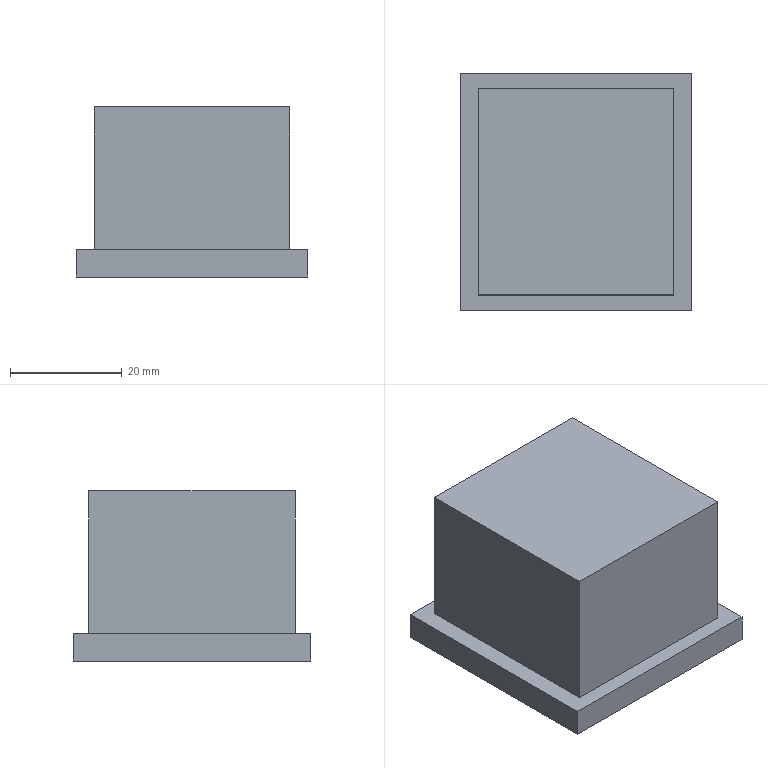Part | NX | features BREP 1 | 1 solid | 40 faces | box 41.6 x 42.6 x 30.5 mm | volume 41782 mm3 | plane 38 | cylinder 2 | commonest cylinder face diameters 2 x2
STEP:
#1=CARTESIAN_POINT('',(20.8,-21.3,0.));
#2=VERTEX_POINT('',#1);
#3=CARTESIAN_POINT('',(20.8,21.3,0.));
#4=VERTEX_POINT('',#3);
#5=CARTESIAN_POINT('',(20.8,-21.3,0.));
#6=DIRECTION('',(0.,1.,0.));
#7=VECTOR('',#6,1000.);
#8=LINE('',#5,#7);
#9=EDGE_CURVE('',#2,#4,#8,.T.);
#10=ORIENTED_EDGE('',*,*,#9,.F.);
#11=CARTESIAN_POINT('',(-20.8,-21.3,0.));
#12=VERTEX_POINT('',#11);
#13=CARTESIAN_POINT('',(-20.8,-21.3,0.));
#14=DIRECTION('',(1.,0.,0.));
#15=VECTOR('',#14,1000.);
#16=LINE('',#13,#15);
#17=EDGE_CURVE('',#12,#2,#16,.T.);
#18=ORIENTED_EDGE('',*,*,#17,.F.);
#19=CARTESIAN_POINT('',(-20.8,21.3,0.));
#20=VERTEX_POINT('',#19);
#21=CARTESIAN_POINT('',(-20.8,21.3,0.));
#22=DIRECTION('',(0.,-1.,0.));
#23=VECTOR('',#22,1000.);
#24=LINE('',#21,#23);
#25=EDGE_CURVE('',#20,#12,#24,.T.);
#26=ORIENTED_EDGE('',*,*,#25,.F.);
#27=CARTESIAN_POINT('',(20.8,21.3,0.));
#28=DIRECTION('',(-1.,0.,0.));
#29=VECTOR('',#28,1000.);
#30=LINE('',#27,#29);
#31=EDGE_CURVE('',#4,#20,#30,.T.);
#32=ORIENTED_EDGE('',*,*,#31,.F.);
#33=EDGE_LOOP('',(#10,#18,#26,#32));
#34=FACE_BOUND('',#33,.T.);
#35=CARTESIAN_POINT('',(3.,5.,0.));
#36=VERTEX_POINT('',#35);
#37=CARTESIAN_POINT('',(3.,8.,0.));
#38=VERTEX_POINT('',#37);
#39=CARTESIAN_POINT('',(3.,5.,0.));
#40=DIRECTION('',(0.,1.,0.));
#41=VECTOR('',#40,1000.);
#42=LINE('',#39,#41);
#43=EDGE_CURVE('',#36,#38,#42,.T.);
#44=ORIENTED_EDGE('',*,*,#43,.F.);
#45=CARTESIAN_POINT('',(3.746,5.,0.));
#46=VERTEX_POINT('',#45);
#47=CARTESIAN_POINT('',(3.746,5.,0.));
#48=DIRECTION('',(-1.,0.,0.));
#49=VECTOR('',#48,1000.);
#50=LINE('',#47,#49);
#51=EDGE_CURVE('',#46,#36,#50,.T.);
#52=ORIENTED_EDGE('',*,*,#51,.F.);
#53=CARTESIAN_POINT('',(3.746,5.609,0.));
#54=VERTEX_POINT('',#53);
#55=CARTESIAN_POINT('',(3.746,5.609,0.));
#56=DIRECTION('',(0.,-1.,0.));
#57=VECTOR('',#56,1000.);
#58=LINE('',#55,#57);
#59=EDGE_CURVE('',#54,#46,#58,.T.);
#60=ORIENTED_EDGE('',*,*,#59,.F.);
#61=CARTESIAN_POINT('',(3.746,7.391,0.));
#62=VERTEX_POINT('',#61);
#63=CARTESIAN_POINT('',(4.2,6.5,0.));
#64=DIRECTION('',(0.,0.,-1.));
#65=DIRECTION('',(-0.4545,0.8908,0.));
#66=AXIS2_PLACEMENT_3D('',#63,#64,#65);
#67=CIRCLE('',#66,1.);
#68=EDGE_CURVE('',#62,#54,#67,.T.);
#69=ORIENTED_EDGE('',*,*,#68,.F.);
#70=CARTESIAN_POINT('',(3.746,8.,0.));
#71=VERTEX_POINT('',#70);
#72=CARTESIAN_POINT('',(3.746,8.,0.));
#73=DIRECTION('',(0.,-1.,0.));
#74=VECTOR('',#73,1000.);
#75=LINE('',#72,#74);
#76=EDGE_CURVE('',#71,#62,#75,.T.);
#77=ORIENTED_EDGE('',*,*,#76,.F.);
#78=CARTESIAN_POINT('',(3.,8.,0.));
#79=DIRECTION('',(1.,0.,0.));
#80=VECTOR('',#79,1000.);
#81=LINE('',#78,#80);
#82=EDGE_CURVE('',#38,#71,#81,.T.);
#83=ORIENTED_EDGE('',*,*,#82,.F.);
#84=EDGE_LOOP('',(#44,#52,#60,#69,#77,#83));
#85=FACE_BOUND('',#84,.T.);
#86=CARTESIAN_POINT('',(-3.746,8.,0.));
#87=VERTEX_POINT('',#86);
#88=CARTESIAN_POINT('',(-3.746,7.391,0.));
#89=VERTEX_POINT('',#88);
#90=CARTESIAN_POINT('',(-3.746,8.,0.));
#91=DIRECTION('',(0.,-1.,0.));
#92=VECTOR('',#91,1000.);
#93=LINE('',#90,#92);
#94=EDGE_CURVE('',#87,#89,#93,.T.);
#95=ORIENTED_EDGE('',*,*,#94,.T.);
#96=CARTESIAN_POINT('',(-3.746,5.609,0.));
#97=VERTEX_POINT('',#96);
#98=CARTESIAN_POINT('',(-4.2,6.5,0.));
#99=DIRECTION('',(0.,0.,1.));
#100=DIRECTION('',(0.4545,0.8908,0.));
#101=AXIS2_PLACEMENT_3D('',#98,#99,#100);
#102=CIRCLE('',#101,1.);
#103=EDGE_CURVE('',#89,#97,#102,.T.);
#104=ORIENTED_EDGE('',*,*,#103,.T.);
#105=CARTESIAN_POINT('',(-3.746,5.,0.));
#106=VERTEX_POINT('',#105);
#107=CARTESIAN_POINT('',(-3.746,5.609,0.));
#108=DIRECTION('',(0.,-1.,0.));
#109=VECTOR('',#108,1000.);
#110=LINE('',#107,#109);
#111=EDGE_CURVE('',#97,#106,#110,.T.);
#112=ORIENTED_EDGE('',*,*,#111,.T.);
#113=CARTESIAN_POINT('',(-3.,5.,0.));
#114=VERTEX_POINT('',#113);
#115=CARTESIAN_POINT('',(-3.746,5.,0.));
#116=DIRECTION('',(1.,0.,0.));
#117=VECTOR('',#116,1000.);
#118=LINE('',#115,#117);
#119=EDGE_CURVE('',#106,#114,#118,.T.);
#120=ORIENTED_EDGE('',*,*,#119,.T.);
#121=CARTESIAN_POINT('',(-3.,8.,0.));
#122=VERTEX_POINT('',#121);
#123=CARTESIAN_POINT('',(-3.,5.,0.));
#124=DIRECTION('',(0.,1.,0.));
#125=VECTOR('',#124,1000.);
#126=LINE('',#123,#125);
#127=EDGE_CURVE('',#114,#122,#126,.T.);
#128=ORIENTED_EDGE('',*,*,#127,.T.);
#129=CARTESIAN_POINT('',(-3.,8.,0.));
#130=DIRECTION('',(-1.,0.,0.));
#131=VECTOR('',#130,1000.);
#132=LINE('',#129,#131);
#133=EDGE_CURVE('',#122,#87,#132,.T.);
#134=ORIENTED_EDGE('',*,*,#133,.T.);
#135=EDGE_LOOP('',(#95,#104,#112,#120,#128,#134));
#136=FACE_BOUND('',#135,.T.);
#137=CARTESIAN_POINT('',(-0.5,5.,0.));
#138=VERTEX_POINT('',#137);
#139=CARTESIAN_POINT('',(-0.5,8.,0.));
#140=VERTEX_POINT('',#139);
#141=CARTESIAN_POINT('',(-0.5,5.,0.));
#142=DIRECTION('',(0.,1.,0.));
#143=VECTOR('',#142,1000.);
#144=LINE('',#141,#143);
#145=EDGE_CURVE('',#138,#140,#144,.T.);
#146=ORIENTED_EDGE('',*,*,#145,.F.);
#147=CARTESIAN_POINT('',(0.5,5.,0.));
#148=VERTEX_POINT('',#147);
#149=CARTESIAN_POINT('',(0.5,5.,0.));
#150=DIRECTION('',(-1.,0.,0.));
#151=VECTOR('',#150,1000.);
#152=LINE('',#149,#151);
#153=EDGE_CURVE('',#148,#138,#152,.T.);
#154=ORIENTED_EDGE('',*,*,#153,.F.);
#155=CARTESIAN_POINT('',(0.5,8.,0.));
#156=VERTEX_POINT('',#155);
#157=CARTESIAN_POINT('',(0.5,8.,0.));
#158=DIRECTION('',(0.,-1.,0.));
#159=VECTOR('',#158,1000.);
#160=LINE('',#157,#159);
#161=EDGE_CURVE('',#156,#148,#160,.T.);
#162=ORIENTED_EDGE('',*,*,#161,.F.);
#163=CARTESIAN_POINT('',(-0.5,8.,0.));
#164=DIRECTION('',(1.,0.,0.));
#165=VECTOR('',#164,1000.);
#166=LINE('',#163,#165);
#167=EDGE_CURVE('',#140,#156,#166,.T.);
#168=ORIENTED_EDGE('',*,*,#167,.F.);
#169=EDGE_LOOP('',(#146,#154,#162,#168));
#170=FACE_BOUND('',#169,.T.);
#171=CARTESIAN_POINT('',(4.299,-2.402,0.));
#172=VERTEX_POINT('',#171);
#173=CARTESIAN_POINT('',(3.298,-1.833,0.));
#174=VERTEX_POINT('',#173);
#175=CARTESIAN_POINT('',(4.299,-2.402,0.));
#176=DIRECTION('',(-0.8695,0.494,0.));
#177=VECTOR('',#176,1000.);
#178=LINE('',#175,#177);
#179=EDGE_CURVE('',#172,#174,#178,.T.);
#180=ORIENTED_EDGE('',*,*,#179,.F.);
#181=CARTESIAN_POINT('',(5.994,0.58,0.));
#182=VERTEX_POINT('',#181);
#183=CARTESIAN_POINT('',(5.994,0.58,0.));
#184=DIRECTION('',(-0.494,-0.8695,0.));
#185=VECTOR('',#184,1000.);
#186=LINE('',#183,#185);
#187=EDGE_CURVE('',#182,#172,#186,.T.);
#188=ORIENTED_EDGE('',*,*,#187,.F.);
#189=CARTESIAN_POINT('',(4.992,1.149,0.));
#190=VERTEX_POINT('',#189);
#191=CARTESIAN_POINT('',(4.992,1.149,0.));
#192=DIRECTION('',(0.8695,-0.494,0.));
#193=VECTOR('',#192,1000.);
#194=LINE('',#191,#193);
#195=EDGE_CURVE('',#190,#182,#194,.T.);
#196=ORIENTED_EDGE('',*,*,#195,.F.);
#197=CARTESIAN_POINT('',(3.298,-1.833,0.));
#198=DIRECTION('',(0.494,0.8695,0.));
#199=VECTOR('',#198,1000.);
#200=LINE('',#197,#199);
#201=EDGE_CURVE('',#174,#190,#200,.T.);
#202=ORIENTED_EDGE('',*,*,#201,.F.);
#203=EDGE_LOOP('',(#180,#188,#196,#202));
#204=FACE_BOUND('',#203,.T.);
#205=CARTESIAN_POINT('',(-4.992,1.149,0.));
#206=VERTEX_POINT('',#205);
#207=CARTESIAN_POINT('',(-5.994,0.58,0.));
#208=VERTEX_POINT('',#207);
#209=CARTESIAN_POINT('',(-4.992,1.149,0.));
#210=DIRECTION('',(-0.8695,-0.494,0.));
#211=VECTOR('',#210,1000.);
#212=LINE('',#209,#211);
#213=EDGE_CURVE('',#206,#208,#212,.T.);
#214=ORIENTED_EDGE('',*,*,#213,.T.);
#215=CARTESIAN_POINT('',(-4.299,-2.402,0.));
#216=VERTEX_POINT('',#215);
#217=CARTESIAN_POINT('',(-5.994,0.58,0.));
#218=DIRECTION('',(0.494,-0.8695,0.));
#219=VECTOR('',#218,1000.);
#220=LINE('',#217,#219);
#221=EDGE_CURVE('',#208,#216,#220,.T.);
#222=ORIENTED_EDGE('',*,*,#221,.T.);
#223=CARTESIAN_POINT('',(-3.298,-1.833,0.));
#224=VERTEX_POINT('',#223);
#225=CARTESIAN_POINT('',(-4.299,-2.402,0.));
#226=DIRECTION('',(0.8695,0.494,0.));
#227=VECTOR('',#226,1000.);
#228=LINE('',#225,#227);
#229=EDGE_CURVE('',#216,#224,#228,.T.);
#230=ORIENTED_EDGE('',*,*,#229,.T.);
#231=CARTESIAN_POINT('',(-3.298,-1.833,0.));
#232=DIRECTION('',(-0.494,0.8695,0.));
#233=VECTOR('',#232,1000.);
#234=LINE('',#231,#233);
#235=EDGE_CURVE('',#224,#206,#234,.T.);
#236=ORIENTED_EDGE('',*,*,#235,.T.);
#237=EDGE_LOOP('',(#214,#222,#230,#236));
#238=FACE_BOUND('',#237,.T.);
#239=CARTESIAN_POINT('',(0.,0.,0.));
#240=DIRECTION('',(0.,0.,1.));
#241=DIRECTION('',(1.,0.,0.));
#242=AXIS2_PLACEMENT_3D('',#239,#240,#241);
#243=PLANE('',#242);
#244=ADVANCED_FACE('',(#34,#85,#136,#170,#204,#238),#243,.F.);
#245=CARTESIAN_POINT('',(-20.8,21.3,5.));
#246=VERTEX_POINT('',#245);
#247=CARTESIAN_POINT('',(-20.8,21.3,0.));
#248=DIRECTION('',(0.,0.,1.));
#249=VECTOR('',#248,1000.);
#250=LINE('',#247,#249);
#251=EDGE_CURVE('',#20,#246,#250,.T.);
#252=ORIENTED_EDGE('',*,*,#251,.T.);
#253=CARTESIAN_POINT('',(20.8,21.3,5.));
#254=VERTEX_POINT('',#253);
#255=CARTESIAN_POINT('',(20.8,21.3,5.));
#256=DIRECTION('',(-1.,0.,0.));
#257=VECTOR('',#256,1000.);
#258=LINE('',#255,#257);
#259=EDGE_CURVE('',#254,#246,#258,.T.);
#260=ORIENTED_EDGE('',*,*,#259,.F.);
#261=CARTESIAN_POINT('',(20.8,21.3,0.));
#262=DIRECTION('',(0.,0.,1.));
#263=VECTOR('',#262,1000.);
#264=LINE('',#261,#263);
#265=EDGE_CURVE('',#4,#254,#264,.T.);
#266=ORIENTED_EDGE('',*,*,#265,.F.);
#267=ORIENTED_EDGE('',*,*,#31,.T.);
#268=EDGE_LOOP('',(#252,#260,#266,#267));
#269=FACE_BOUND('',#268,.T.);
#270=CARTESIAN_POINT('',(20.8,21.3,0.));
#271=DIRECTION('',(0.,1.,0.));
#272=DIRECTION('',(1.,0.,0.));
#273=AXIS2_PLACEMENT_3D('',#270,#271,#272);
#274=PLANE('',#273);
#275=ADVANCED_FACE('',(#269),#274,.T.);
#276=ORIENTED_EDGE('',*,*,#265,.T.);
#277=CARTESIAN_POINT('',(20.8,-21.3,5.));
#278=VERTEX_POINT('',#277);
#279=CARTESIAN_POINT('',(20.8,-21.3,5.));
#280=DIRECTION('',(0.,1.,0.));
#281=VECTOR('',#280,1000.);
#282=LINE('',#279,#281);
#283=EDGE_CURVE('',#278,#254,#282,.T.);
#284=ORIENTED_EDGE('',*,*,#283,.F.);
#285=CARTESIAN_POINT('',(20.8,-21.3,0.));
#286=DIRECTION('',(0.,0.,1.));
#287=VECTOR('',#286,1000.);
#288=LINE('',#285,#287);
#289=EDGE_CURVE('',#2,#278,#288,.T.);
#290=ORIENTED_EDGE('',*,*,#289,.F.);
#291=ORIENTED_EDGE('',*,*,#9,.T.);
#292=EDGE_LOOP('',(#276,#284,#290,#291));
#293=FACE_BOUND('',#292,.T.);
#294=CARTESIAN_POINT('',(20.8,-21.3,0.));
#295=DIRECTION('',(1.,0.,0.));
#296=DIRECTION('',(0.,1.,0.));
#297=AXIS2_PLACEMENT_3D('',#294,#295,#296);
#298=PLANE('',#297);
#299=ADVANCED_FACE('',(#293),#298,.T.);
#300=ORIENTED_EDGE('',*,*,#289,.T.);
#301=CARTESIAN_POINT('',(-20.8,-21.3,5.));
#302=VERTEX_POINT('',#301);
#303=CARTESIAN_POINT('',(-20.8,-21.3,5.));
#304=DIRECTION('',(1.,0.,0.));
#305=VECTOR('',#304,1000.);
#306=LINE('',#303,#305);
#307=EDGE_CURVE('',#302,#278,#306,.T.);
#308=ORIENTED_EDGE('',*,*,#307,.F.);
#309=CARTESIAN_POINT('',(-20.8,-21.3,0.));
#310=DIRECTION('',(0.,0.,1.));
#311=VECTOR('',#310,1000.);
#312=LINE('',#309,#311);
#313=EDGE_CURVE('',#12,#302,#312,.T.);
#314=ORIENTED_EDGE('',*,*,#313,.F.);
#315=ORIENTED_EDGE('',*,*,#17,.T.);
#316=EDGE_LOOP('',(#300,#308,#314,#315));
#317=FACE_BOUND('',#316,.T.);
#318=CARTESIAN_POINT('',(-20.8,-21.3,0.));
#319=DIRECTION('',(0.,-1.,0.));
#320=DIRECTION('',(0.,0.,-1.));
#321=AXIS2_PLACEMENT_3D('',#318,#319,#320);
#322=PLANE('',#321);
#323=ADVANCED_FACE('',(#317),#322,.T.);
#324=ORIENTED_EDGE('',*,*,#313,.T.);
#325=CARTESIAN_POINT('',(-20.8,21.3,5.));
#326=DIRECTION('',(0.,-1.,0.));
#327=VECTOR('',#326,1000.);
#328=LINE('',#325,#327);
#329=EDGE_CURVE('',#246,#302,#328,.T.);
#330=ORIENTED_EDGE('',*,*,#329,.F.);
#331=ORIENTED_EDGE('',*,*,#251,.F.);
#332=ORIENTED_EDGE('',*,*,#25,.T.);
#333=EDGE_LOOP('',(#324,#330,#331,#332));
#334=FACE_BOUND('',#333,.T.);
#335=CARTESIAN_POINT('',(-20.8,21.3,0.));
#336=DIRECTION('',(-1.,0.,0.));
#337=DIRECTION('',(0.,0.,1.));
#338=AXIS2_PLACEMENT_3D('',#335,#336,#337);
#339=PLANE('',#338);
#340=ADVANCED_FACE('',(#334),#339,.T.);
#341=ORIENTED_EDGE('',*,*,#329,.T.);
#342=ORIENTED_EDGE('',*,*,#307,.T.);
#343=ORIENTED_EDGE('',*,*,#283,.T.);
#344=ORIENTED_EDGE('',*,*,#259,.T.);
#345=EDGE_LOOP('',(#341,#342,#343,#344));
#346=FACE_BOUND('',#345,.T.);
#347=CARTESIAN_POINT('',(17.5,18.5,5.));
#348=VERTEX_POINT('',#347);
#349=CARTESIAN_POINT('',(-17.5,18.5,5.));
#350=VERTEX_POINT('',#349);
#351=CARTESIAN_POINT('',(17.5,18.5,5.));
#352=DIRECTION('',(-1.,0.,0.));
#353=VECTOR('',#352,1000.);
#354=LINE('',#351,#353);
#355=EDGE_CURVE('',#348,#350,#354,.T.);
#356=ORIENTED_EDGE('',*,*,#355,.F.);
#357=CARTESIAN_POINT('',(17.5,-18.5,5.));
#358=VERTEX_POINT('',#357);
#359=CARTESIAN_POINT('',(17.5,-18.5,5.));
#360=DIRECTION('',(0.,1.,0.));
#361=VECTOR('',#360,1000.);
#362=LINE('',#359,#361);
#363=EDGE_CURVE('',#358,#348,#362,.T.);
#364=ORIENTED_EDGE('',*,*,#363,.F.);
#365=CARTESIAN_POINT('',(-17.5,-18.5,5.));
#366=VERTEX_POINT('',#365);
#367=CARTESIAN_POINT('',(-17.5,-18.5,5.));
#368=DIRECTION('',(1.,0.,0.));
#369=VECTOR('',#368,1000.);
#370=LINE('',#367,#369);
#371=EDGE_CURVE('',#366,#358,#370,.T.);
#372=ORIENTED_EDGE('',*,*,#371,.F.);
#373=CARTESIAN_POINT('',(-17.5,18.5,5.));
#374=DIRECTION('',(0.,-1.,0.));
#375=VECTOR('',#374,1000.);
#376=LINE('',#373,#375);
#377=EDGE_CURVE('',#350,#366,#376,.T.);
#378=ORIENTED_EDGE('',*,*,#377,.F.);
#379=EDGE_LOOP('',(#356,#364,#372,#378));
#380=FACE_BOUND('',#379,.T.);
#381=CARTESIAN_POINT('',(0.,0.,5.));
#382=DIRECTION('',(0.,0.,1.));
#383=DIRECTION('',(1.,0.,0.));
#384=AXIS2_PLACEMENT_3D('',#381,#382,#383);
#385=PLANE('',#384);
#386=ADVANCED_FACE('',(#346,#380),#385,.T.);
#387=CARTESIAN_POINT('',(-17.5,-18.5,30.5));
#388=VERTEX_POINT('',#387);
#389=CARTESIAN_POINT('',(-17.5,-18.5,5.));
#390=DIRECTION('',(0.,0.,1.));
#391=VECTOR('',#390,1000.);
#392=LINE('',#389,#391);
#393=EDGE_CURVE('',#366,#388,#392,.T.);
#394=ORIENTED_EDGE('',*,*,#393,.T.);
#395=CARTESIAN_POINT('',(-17.5,18.5,30.5));
#396=VERTEX_POINT('',#395);
#397=CARTESIAN_POINT('',(-17.5,18.5,30.5));
#398=DIRECTION('',(0.,-1.,0.));
#399=VECTOR('',#398,1000.);
#400=LINE('',#397,#399);
#401=EDGE_CURVE('',#396,#388,#400,.T.);
#402=ORIENTED_EDGE('',*,*,#401,.F.);
#403=CARTESIAN_POINT('',(-17.5,18.5,5.));
#404=DIRECTION('',(0.,0.,1.));
#405=VECTOR('',#404,1000.);
#406=LINE('',#403,#405);
#407=EDGE_CURVE('',#350,#396,#406,.T.);
#408=ORIENTED_EDGE('',*,*,#407,.F.);
#409=ORIENTED_EDGE('',*,*,#377,.T.);
#410=EDGE_LOOP('',(#394,#402,#408,#409));
#411=FACE_BOUND('',#410,.T.);
#412=CARTESIAN_POINT('',(-17.5,18.5,5.));
#413=DIRECTION('',(-1.,0.,0.));
#414=DIRECTION('',(0.,0.,1.));
#415=AXIS2_PLACEMENT_3D('',#412,#413,#414);
#416=PLANE('',#415);
#417=ADVANCED_FACE('',(#411),#416,.T.);
#418=ORIENTED_EDGE('',*,*,#407,.T.);
#419=CARTESIAN_POINT('',(17.5,18.5,30.5));
#420=VERTEX_POINT('',#419);
#421=CARTESIAN_POINT('',(17.5,18.5,30.5));
#422=DIRECTION('',(-1.,0.,0.));
#423=VECTOR('',#422,1000.);
#424=LINE('',#421,#423);
#425=EDGE_CURVE('',#420,#396,#424,.T.);
#426=ORIENTED_EDGE('',*,*,#425,.F.);
#427=CARTESIAN_POINT('',(17.5,18.5,5.));
#428=DIRECTION('',(0.,0.,1.));
#429=VECTOR('',#428,1000.);
#430=LINE('',#427,#429);
#431=EDGE_CURVE('',#348,#420,#430,.T.);
#432=ORIENTED_EDGE('',*,*,#431,.F.);
#433=ORIENTED_EDGE('',*,*,#355,.T.);
#434=EDGE_LOOP('',(#418,#426,#432,#433));
#435=FACE_BOUND('',#434,.T.);
#436=CARTESIAN_POINT('',(17.5,18.5,5.));
#437=DIRECTION('',(0.,1.,0.));
#438=DIRECTION('',(1.,0.,0.));
#439=AXIS2_PLACEMENT_3D('',#436,#437,#438);
#440=PLANE('',#439);
#441=ADVANCED_FACE('',(#435),#440,.T.);
#442=ORIENTED_EDGE('',*,*,#431,.T.);
#443=CARTESIAN_POINT('',(17.5,-18.5,30.5));
#444=VERTEX_POINT('',#443);
#445=CARTESIAN_POINT('',(17.5,-18.5,30.5));
#446=DIRECTION('',(0.,1.,0.));
#447=VECTOR('',#446,1000.);
#448=LINE('',#445,#447);
#449=EDGE_CURVE('',#444,#420,#448,.T.);
#450=ORIENTED_EDGE('',*,*,#449,.F.);
#451=CARTESIAN_POINT('',(17.5,-18.5,5.));
#452=DIRECTION('',(0.,0.,1.));
#453=VECTOR('',#452,1000.);
#454=LINE('',#451,#453);
#455=EDGE_CURVE('',#358,#444,#454,.T.);
#456=ORIENTED_EDGE('',*,*,#455,.F.);
#457=ORIENTED_EDGE('',*,*,#363,.T.);
#458=EDGE_LOOP('',(#442,#450,#456,#457));
#459=FACE_BOUND('',#458,.T.);
#460=CARTESIAN_POINT('',(17.5,-18.5,5.));
#461=DIRECTION('',(1.,0.,0.));
#462=DIRECTION('',(0.,1.,0.));
#463=AXIS2_PLACEMENT_3D('',#460,#461,#462);
#464=PLANE('',#463);
#465=ADVANCED_FACE('',(#459),#464,.T.);
#466=ORIENTED_EDGE('',*,*,#455,.T.);
#467=CARTESIAN_POINT('',(-17.5,-18.5,30.5));
#468=DIRECTION('',(1.,0.,0.));
#469=VECTOR('',#468,1000.);
#470=LINE('',#467,#469);
#471=EDGE_CURVE('',#388,#444,#470,.T.);
#472=ORIENTED_EDGE('',*,*,#471,.F.);
#473=ORIENTED_EDGE('',*,*,#393,.F.);
#474=ORIENTED_EDGE('',*,*,#371,.T.);
#475=EDGE_LOOP('',(#466,#472,#473,#474));
#476=FACE_BOUND('',#475,.T.);
#477=CARTESIAN_POINT('',(-17.5,-18.5,5.));
#478=DIRECTION('',(0.,-1.,0.));
#479=DIRECTION('',(0.,0.,-1.));
#480=AXIS2_PLACEMENT_3D('',#477,#478,#479);
#481=PLANE('',#480);
#482=ADVANCED_FACE('',(#476),#481,.T.);
#483=ORIENTED_EDGE('',*,*,#471,.T.);
#484=ORIENTED_EDGE('',*,*,#449,.T.);
#485=ORIENTED_EDGE('',*,*,#425,.T.);
#486=ORIENTED_EDGE('',*,*,#401,.T.);
#487=EDGE_LOOP('',(#483,#484,#485,#486));
#488=FACE_BOUND('',#487,.T.);
#489=CARTESIAN_POINT('',(0.,0.,30.5));
#490=DIRECTION('',(0.,0.,1.));
#491=DIRECTION('',(1.,0.,0.));
#492=AXIS2_PLACEMENT_3D('',#489,#490,#491);
#493=PLANE('',#492);
#494=ADVANCED_FACE('',(#488),#493,.T.);
#495=CARTESIAN_POINT('',(3.746,8.,5.));
#496=VERTEX_POINT('',#495);
#497=CARTESIAN_POINT('',(3.746,8.,0.));
#498=DIRECTION('',(0.,0.,1.));
#499=VECTOR('',#498,1000.);
#500=LINE('',#497,#499);
#501=EDGE_CURVE('',#71,#496,#500,.T.);
#502=ORIENTED_EDGE('',*,*,#501,.T.);
#503=CARTESIAN_POINT('',(3.,8.,5.));
#504=VERTEX_POINT('',#503);
#505=CARTESIAN_POINT('',(3.,8.,5.));
#506=DIRECTION('',(1.,0.,0.));
#507=VECTOR('',#506,1000.);
#508=LINE('',#505,#507);
#509=EDGE_CURVE('',#504,#496,#508,.T.);
#510=ORIENTED_EDGE('',*,*,#509,.F.);
#511=CARTESIAN_POINT('',(3.,8.,0.));
#512=DIRECTION('',(0.,0.,1.));
#513=VECTOR('',#512,1000.);
#514=LINE('',#511,#513);
#515=EDGE_CURVE('',#38,#504,#514,.T.);
#516=ORIENTED_EDGE('',*,*,#515,.F.);
#517=ORIENTED_EDGE('',*,*,#82,.T.);
#518=EDGE_LOOP('',(#502,#510,#516,#517));
#519=FACE_BOUND('',#518,.T.);
#520=CARTESIAN_POINT('',(3.,8.,0.));
#521=DIRECTION('',(0.,1.,0.));
#522=DIRECTION('',(1.,0.,0.));
#523=AXIS2_PLACEMENT_3D('',#520,#521,#522);
#524=PLANE('',#523);
#525=ADVANCED_FACE('',(#519),#524,.F.);
#526=ORIENTED_EDGE('',*,*,#515,.T.);
#527=CARTESIAN_POINT('',(3.,5.,5.));
#528=VERTEX_POINT('',#527);
#529=CARTESIAN_POINT('',(3.,5.,5.));
#530=DIRECTION('',(0.,1.,0.));
#531=VECTOR('',#530,1000.);
#532=LINE('',#529,#531);
#533=EDGE_CURVE('',#528,#504,#532,.T.);
#534=ORIENTED_EDGE('',*,*,#533,.F.);
#535=CARTESIAN_POINT('',(3.,5.,0.));
#536=DIRECTION('',(0.,0.,1.));
#537=VECTOR('',#536,1000.);
#538=LINE('',#535,#537);
#539=EDGE_CURVE('',#36,#528,#538,.T.);
#540=ORIENTED_EDGE('',*,*,#539,.F.);
#541=ORIENTED_EDGE('',*,*,#43,.T.);
#542=EDGE_LOOP('',(#526,#534,#540,#541));
#543=FACE_BOUND('',#542,.T.);
#544=CARTESIAN_POINT('',(3.,5.,0.));
#545=DIRECTION('',(-1.,0.,0.));
#546=DIRECTION('',(0.,0.,1.));
#547=AXIS2_PLACEMENT_3D('',#544,#545,#546);
#548=PLANE('',#547);
#549=ADVANCED_FACE('',(#543),#548,.F.);
#550=ORIENTED_EDGE('',*,*,#539,.T.);
#551=CARTESIAN_POINT('',(3.746,5.,5.));
#552=VERTEX_POINT('',#551);
#553=CARTESIAN_POINT('',(3.746,5.,5.));
#554=DIRECTION('',(-1.,0.,0.));
#555=VECTOR('',#554,1000.);
#556=LINE('',#553,#555);
#557=EDGE_CURVE('',#552,#528,#556,.T.);
#558=ORIENTED_EDGE('',*,*,#557,.F.);
#559=CARTESIAN_POINT('',(3.746,5.,0.));
#560=DIRECTION('',(0.,0.,1.));
#561=VECTOR('',#560,1000.);
#562=LINE('',#559,#561);
#563=EDGE_CURVE('',#46,#552,#562,.T.);
#564=ORIENTED_EDGE('',*,*,#563,.F.);
#565=ORIENTED_EDGE('',*,*,#51,.T.);
#566=EDGE_LOOP('',(#550,#558,#564,#565));
#567=FACE_BOUND('',#566,.T.);
#568=CARTESIAN_POINT('',(3.746,5.,0.));
#569=DIRECTION('',(0.,-1.,0.));
#570=DIRECTION('',(0.,0.,-1.));
#571=AXIS2_PLACEMENT_3D('',#568,#569,#570);
#572=PLANE('',#571);
#573=ADVANCED_FACE('',(#567),#572,.F.);
#574=ORIENTED_EDGE('',*,*,#563,.T.);
#575=CARTESIAN_POINT('',(3.746,5.609,5.));
#576=VERTEX_POINT('',#575);
#577=CARTESIAN_POINT('',(3.746,5.609,5.));
#578=DIRECTION('',(0.,-1.,0.));
#579=VECTOR('',#578,1000.);
#580=LINE('',#577,#579);
#581=EDGE_CURVE('',#576,#552,#580,.T.);
#582=ORIENTED_EDGE('',*,*,#581,.F.);
#583=CARTESIAN_POINT('',(3.746,5.609,0.));
#584=DIRECTION('',(0.,0.,1.));
#585=VECTOR('',#584,1000.);
#586=LINE('',#583,#585);
#587=EDGE_CURVE('',#54,#576,#586,.T.);
#588=ORIENTED_EDGE('',*,*,#587,.F.);
#589=ORIENTED_EDGE('',*,*,#59,.T.);
#590=EDGE_LOOP('',(#574,#582,#588,#589));
#591=FACE_BOUND('',#590,.T.);
#592=CARTESIAN_POINT('',(3.746,5.609,0.));
#593=DIRECTION('',(1.,0.,0.));
#594=DIRECTION('',(0.,1.,0.));
#595=AXIS2_PLACEMENT_3D('',#592,#593,#594);
#596=PLANE('',#595);
#597=ADVANCED_FACE('',(#591),#596,.F.);
#598=ORIENTED_EDGE('',*,*,#587,.T.);
#599=CARTESIAN_POINT('',(3.746,7.391,5.));
#600=VERTEX_POINT('',#599);
#601=CARTESIAN_POINT('',(4.2,6.5,5.));
#602=DIRECTION('',(0.,0.,-1.));
#603=DIRECTION('',(-0.4545,0.8908,0.));
#604=AXIS2_PLACEMENT_3D('',#601,#602,#603);
#605=CIRCLE('',#604,1.);
#606=EDGE_CURVE('',#600,#576,#605,.T.);
#607=ORIENTED_EDGE('',*,*,#606,.F.);
#608=CARTESIAN_POINT('',(3.746,7.391,0.));
#609=DIRECTION('',(0.,0.,1.));
#610=VECTOR('',#609,1000.);
#611=LINE('',#608,#610);
#612=EDGE_CURVE('',#62,#600,#611,.T.);
#613=ORIENTED_EDGE('',*,*,#612,.F.);
#614=ORIENTED_EDGE('',*,*,#68,.T.);
#615=EDGE_LOOP('',(#598,#607,#613,#614));
#616=FACE_BOUND('',#615,.T.);
#617=CARTESIAN_POINT('',(4.2,6.5,0.));
#618=DIRECTION('',(0.,0.,-1.));
#619=DIRECTION('',(-1.,0.,0.));
#620=AXIS2_PLACEMENT_3D('',#617,#618,#619);
#621=CYLINDRICAL_SURFACE('',#620,1.);
#622=ADVANCED_FACE('',(#616),#621,.F.);
#623=ORIENTED_EDGE('',*,*,#612,.T.);
#624=CARTESIAN_POINT('',(3.746,8.,5.));
#625=DIRECTION('',(0.,-1.,0.));
#626=VECTOR('',#625,1000.);
#627=LINE('',#624,#626);
#628=EDGE_CURVE('',#496,#600,#627,.T.);
#629=ORIENTED_EDGE('',*,*,#628,.F.);
#630=ORIENTED_EDGE('',*,*,#501,.F.);
#631=ORIENTED_EDGE('',*,*,#76,.T.);
#632=EDGE_LOOP('',(#623,#629,#630,#631));
#633=FACE_BOUND('',#632,.T.);
#634=CARTESIAN_POINT('',(3.746,8.,0.));
#635=DIRECTION('',(1.,0.,0.));
#636=DIRECTION('',(0.,1.,0.));
#637=AXIS2_PLACEMENT_3D('',#634,#635,#636);
#638=PLANE('',#637);
#639=ADVANCED_FACE('',(#633),#638,.F.);
#640=ORIENTED_EDGE('',*,*,#628,.T.);
#641=ORIENTED_EDGE('',*,*,#606,.T.);
#642=ORIENTED_EDGE('',*,*,#581,.T.);
#643=ORIENTED_EDGE('',*,*,#557,.T.);
#644=ORIENTED_EDGE('',*,*,#533,.T.);
#645=ORIENTED_EDGE('',*,*,#509,.T.);
#646=EDGE_LOOP('',(#640,#641,#642,#643,#644,#645));
#647=FACE_BOUND('',#646,.T.);
#648=CARTESIAN_POINT('',(0.,0.,5.));
#649=DIRECTION('',(0.,0.,-1.));
#650=DIRECTION('',(0.,-1.,0.));
#651=AXIS2_PLACEMENT_3D('',#648,#649,#650);
#652=PLANE('',#651);
#653=ADVANCED_FACE('',(#647),#652,.T.);
#654=CARTESIAN_POINT('',(-3.,8.,5.));
#655=VERTEX_POINT('',#654);
#656=CARTESIAN_POINT('',(-3.746,8.,5.));
#657=VERTEX_POINT('',#656);
#658=CARTESIAN_POINT('',(-3.,8.,5.));
#659=DIRECTION('',(-1.,0.,0.));
#660=VECTOR('',#659,1000.);
#661=LINE('',#658,#660);
#662=EDGE_CURVE('',#655,#657,#661,.T.);
#663=ORIENTED_EDGE('',*,*,#662,.T.);
#664=CARTESIAN_POINT('',(-3.746,8.,0.));
#665=DIRECTION('',(0.,0.,1.));
#666=VECTOR('',#665,1000.);
#667=LINE('',#664,#666);
#668=EDGE_CURVE('',#87,#657,#667,.T.);
#669=ORIENTED_EDGE('',*,*,#668,.F.);
#670=ORIENTED_EDGE('',*,*,#133,.F.);
#671=CARTESIAN_POINT('',(-3.,8.,0.));
#672=DIRECTION('',(0.,0.,1.));
#673=VECTOR('',#672,1000.);
#674=LINE('',#671,#673);
#675=EDGE_CURVE('',#122,#655,#674,.T.);
#676=ORIENTED_EDGE('',*,*,#675,.T.);
#677=EDGE_LOOP('',(#663,#669,#670,#676));
#678=FACE_BOUND('',#677,.T.);
#679=CARTESIAN_POINT('',(-3.,8.,0.));
#680=DIRECTION('',(0.,-1.,0.));
#681=DIRECTION('',(0.,0.,-1.));
#682=AXIS2_PLACEMENT_3D('',#679,#680,#681);
#683=PLANE('',#682);
#684=ADVANCED_FACE('',(#678),#683,.T.);
#685=ORIENTED_EDGE('',*,*,#127,.F.);
#686=CARTESIAN_POINT('',(-3.,5.,5.));
#687=VERTEX_POINT('',#686);
#688=CARTESIAN_POINT('',(-3.,5.,0.));
#689=DIRECTION('',(0.,0.,1.));
#690=VECTOR('',#689,1000.);
#691=LINE('',#688,#690);
#692=EDGE_CURVE('',#114,#687,#691,.T.);
#693=ORIENTED_EDGE('',*,*,#692,.T.);
#694=CARTESIAN_POINT('',(-3.,5.,5.));
#695=DIRECTION('',(0.,1.,0.));
#696=VECTOR('',#695,1000.);
#697=LINE('',#694,#696);
#698=EDGE_CURVE('',#687,#655,#697,.T.);
#699=ORIENTED_EDGE('',*,*,#698,.T.);
#700=ORIENTED_EDGE('',*,*,#675,.F.);
#701=EDGE_LOOP('',(#685,#693,#699,#700));
#702=FACE_BOUND('',#701,.T.);
#703=CARTESIAN_POINT('',(-3.,5.,0.));
#704=DIRECTION('',(-1.,0.,0.));
#705=DIRECTION('',(0.,0.,1.));
#706=AXIS2_PLACEMENT_3D('',#703,#704,#705);
#707=PLANE('',#706);
#708=ADVANCED_FACE('',(#702),#707,.T.);
#709=ORIENTED_EDGE('',*,*,#698,.F.);
#710=CARTESIAN_POINT('',(-3.746,5.,5.));
#711=VERTEX_POINT('',#710);
#712=CARTESIAN_POINT('',(-3.746,5.,5.));
#713=DIRECTION('',(1.,0.,0.));
#714=VECTOR('',#713,1000.);
#715=LINE('',#712,#714);
#716=EDGE_CURVE('',#711,#687,#715,.T.);
#717=ORIENTED_EDGE('',*,*,#716,.F.);
#718=CARTESIAN_POINT('',(-3.746,5.609,5.));
#719=VERTEX_POINT('',#718);
#720=CARTESIAN_POINT('',(-3.746,5.609,5.));
#721=DIRECTION('',(0.,-1.,0.));
#722=VECTOR('',#721,1000.);
#723=LINE('',#720,#722);
#724=EDGE_CURVE('',#719,#711,#723,.T.);
#725=ORIENTED_EDGE('',*,*,#724,.F.);
#726=CARTESIAN_POINT('',(-3.746,7.391,5.));
#727=VERTEX_POINT('',#726);
#728=CARTESIAN_POINT('',(-4.2,6.5,5.));
#729=DIRECTION('',(0.,0.,1.));
#730=DIRECTION('',(0.4545,0.8908,0.));
#731=AXIS2_PLACEMENT_3D('',#728,#729,#730);
#732=CIRCLE('',#731,1.);
#733=EDGE_CURVE('',#727,#719,#732,.T.);
#734=ORIENTED_EDGE('',*,*,#733,.F.);
#735=CARTESIAN_POINT('',(-3.746,8.,5.));
#736=DIRECTION('',(0.,-1.,0.));
#737=VECTOR('',#736,1000.);
#738=LINE('',#735,#737);
#739=EDGE_CURVE('',#657,#727,#738,.T.);
#740=ORIENTED_EDGE('',*,*,#739,.F.);
#741=ORIENTED_EDGE('',*,*,#662,.F.);
#742=EDGE_LOOP('',(#709,#717,#725,#734,#740,#741));
#743=FACE_BOUND('',#742,.T.);
#744=CARTESIAN_POINT('',(0.,0.,5.));
#745=DIRECTION('',(0.,0.,1.));
#746=DIRECTION('',(1.,0.,0.));
#747=AXIS2_PLACEMENT_3D('',#744,#745,#746);
#748=PLANE('',#747);
#749=ADVANCED_FACE('',(#743),#748,.F.);
#750=ORIENTED_EDGE('',*,*,#739,.T.);
#751=CARTESIAN_POINT('',(-3.746,7.391,0.));
#752=DIRECTION('',(0.,0.,1.));
#753=VECTOR('',#752,1000.);
#754=LINE('',#751,#753);
#755=EDGE_CURVE('',#89,#727,#754,.T.);
#756=ORIENTED_EDGE('',*,*,#755,.F.);
#757=ORIENTED_EDGE('',*,*,#94,.F.);
#758=ORIENTED_EDGE('',*,*,#668,.T.);
#759=EDGE_LOOP('',(#750,#756,#757,#758));
#760=FACE_BOUND('',#759,.T.);
#761=CARTESIAN_POINT('',(-3.746,8.,0.));
#762=DIRECTION('',(1.,0.,0.));
#763=DIRECTION('',(0.,1.,0.));
#764=AXIS2_PLACEMENT_3D('',#761,#762,#763);
#765=PLANE('',#764);
#766=ADVANCED_FACE('',(#760),#765,.T.);
#767=ORIENTED_EDGE('',*,*,#733,.T.);
#768=CARTESIAN_POINT('',(-3.746,5.609,0.));
#769=DIRECTION('',(0.,0.,1.));
#770=VECTOR('',#769,1000.);
#771=LINE('',#768,#770);
#772=EDGE_CURVE('',#97,#719,#771,.T.);
#773=ORIENTED_EDGE('',*,*,#772,.F.);
#774=ORIENTED_EDGE('',*,*,#103,.F.);
#775=ORIENTED_EDGE('',*,*,#755,.T.);
#776=EDGE_LOOP('',(#767,#773,#774,#775));
#777=FACE_BOUND('',#776,.T.);
#778=CARTESIAN_POINT('',(-4.2,6.5,0.));
#779=DIRECTION('',(0.,0.,1.));
#780=DIRECTION('',(1.,0.,0.));
#781=AXIS2_PLACEMENT_3D('',#778,#779,#780);
#782=CYLINDRICAL_SURFACE('',#781,1.);
#783=ADVANCED_FACE('',(#777),#782,.F.);
#784=ORIENTED_EDGE('',*,*,#724,.T.);
#785=CARTESIAN_POINT('',(-3.746,5.,0.));
#786=DIRECTION('',(0.,0.,1.));
#787=VECTOR('',#786,1000.);
#788=LINE('',#785,#787);
#789=EDGE_CURVE('',#106,#711,#788,.T.);
#790=ORIENTED_EDGE('',*,*,#789,.F.);
#791=ORIENTED_EDGE('',*,*,#111,.F.);
#792=ORIENTED_EDGE('',*,*,#772,.T.);
#793=EDGE_LOOP('',(#784,#790,#791,#792));
#794=FACE_BOUND('',#793,.T.);
#795=CARTESIAN_POINT('',(-3.746,5.609,0.));
#796=DIRECTION('',(1.,0.,0.));
#797=DIRECTION('',(0.,1.,0.));
#798=AXIS2_PLACEMENT_3D('',#795,#796,#797);
#799=PLANE('',#798);
#800=ADVANCED_FACE('',(#794),#799,.T.);
#801=ORIENTED_EDGE('',*,*,#716,.T.);
#802=ORIENTED_EDGE('',*,*,#692,.F.);
#803=ORIENTED_EDGE('',*,*,#119,.F.);
#804=ORIENTED_EDGE('',*,*,#789,.T.);
#805=EDGE_LOOP('',(#801,#802,#803,#804));
#806=FACE_BOUND('',#805,.T.);
#807=CARTESIAN_POINT('',(-3.746,5.,0.));
#808=DIRECTION('',(0.,1.,0.));
#809=DIRECTION('',(1.,0.,0.));
#810=AXIS2_PLACEMENT_3D('',#807,#808,#809);
#811=PLANE('',#810);
#812=ADVANCED_FACE('',(#806),#811,.T.);
#813=CARTESIAN_POINT('',(0.5,8.,5.));
#814=VERTEX_POINT('',#813);
#815=CARTESIAN_POINT('',(0.5,8.,0.));
#816=DIRECTION('',(0.,0.,1.));
#817=VECTOR('',#816,1000.);
#818=LINE('',#815,#817);
#819=EDGE_CURVE('',#156,#814,#818,.T.);
#820=ORIENTED_EDGE('',*,*,#819,.T.);
#821=CARTESIAN_POINT('',(-0.5,8.,5.));
#822=VERTEX_POINT('',#821);
#823=CARTESIAN_POINT('',(-0.5,8.,5.));
#824=DIRECTION('',(1.,0.,0.));
#825=VECTOR('',#824,1000.);
#826=LINE('',#823,#825);
#827=EDGE_CURVE('',#822,#814,#826,.T.);
#828=ORIENTED_EDGE('',*,*,#827,.F.);
#829=CARTESIAN_POINT('',(-0.5,8.,0.));
#830=DIRECTION('',(0.,0.,1.));
#831=VECTOR('',#830,1000.);
#832=LINE('',#829,#831);
#833=EDGE_CURVE('',#140,#822,#832,.T.);
#834=ORIENTED_EDGE('',*,*,#833,.F.);
#835=ORIENTED_EDGE('',*,*,#167,.T.);
#836=EDGE_LOOP('',(#820,#828,#834,#835));
#837=FACE_BOUND('',#836,.T.);
#838=CARTESIAN_POINT('',(-0.5,8.,0.));
#839=DIRECTION('',(0.,1.,0.));
#840=DIRECTION('',(1.,0.,0.));
#841=AXIS2_PLACEMENT_3D('',#838,#839,#840);
#842=PLANE('',#841);
#843=ADVANCED_FACE('',(#837),#842,.F.);
#844=ORIENTED_EDGE('',*,*,#833,.T.);
#845=CARTESIAN_POINT('',(-0.5,5.,5.));
#846=VERTEX_POINT('',#845);
#847=CARTESIAN_POINT('',(-0.5,5.,5.));
#848=DIRECTION('',(0.,1.,0.));
#849=VECTOR('',#848,1000.);
#850=LINE('',#847,#849);
#851=EDGE_CURVE('',#846,#822,#850,.T.);
#852=ORIENTED_EDGE('',*,*,#851,.F.);
#853=CARTESIAN_POINT('',(-0.5,5.,0.));
#854=DIRECTION('',(0.,0.,1.));
#855=VECTOR('',#854,1000.);
#856=LINE('',#853,#855);
#857=EDGE_CURVE('',#138,#846,#856,.T.);
#858=ORIENTED_EDGE('',*,*,#857,.F.);
#859=ORIENTED_EDGE('',*,*,#145,.T.);
#860=EDGE_LOOP('',(#844,#852,#858,#859));
#861=FACE_BOUND('',#860,.T.);
#862=CARTESIAN_POINT('',(-0.5,5.,0.));
#863=DIRECTION('',(-1.,0.,0.));
#864=DIRECTION('',(0.,0.,1.));
#865=AXIS2_PLACEMENT_3D('',#862,#863,#864);
#866=PLANE('',#865);
#867=ADVANCED_FACE('',(#861),#866,.F.);
#868=ORIENTED_EDGE('',*,*,#857,.T.);
#869=CARTESIAN_POINT('',(0.5,5.,5.));
#870=VERTEX_POINT('',#869);
#871=CARTESIAN_POINT('',(0.5,5.,5.));
#872=DIRECTION('',(-1.,0.,0.));
#873=VECTOR('',#872,1000.);
#874=LINE('',#871,#873);
#875=EDGE_CURVE('',#870,#846,#874,.T.);
#876=ORIENTED_EDGE('',*,*,#875,.F.);
#877=CARTESIAN_POINT('',(0.5,5.,0.));
#878=DIRECTION('',(0.,0.,1.));
#879=VECTOR('',#878,1000.);
#880=LINE('',#877,#879);
#881=EDGE_CURVE('',#148,#870,#880,.T.);
#882=ORIENTED_EDGE('',*,*,#881,.F.);
#883=ORIENTED_EDGE('',*,*,#153,.T.);
#884=EDGE_LOOP('',(#868,#876,#882,#883));
#885=FACE_BOUND('',#884,.T.);
#886=CARTESIAN_POINT('',(0.5,5.,0.));
#887=DIRECTION('',(0.,-1.,0.));
#888=DIRECTION('',(0.,0.,-1.));
#889=AXIS2_PLACEMENT_3D('',#886,#887,#888);
#890=PLANE('',#889);
#891=ADVANCED_FACE('',(#885),#890,.F.);
#892=ORIENTED_EDGE('',*,*,#881,.T.);
#893=CARTESIAN_POINT('',(0.5,8.,5.));
#894=DIRECTION('',(0.,-1.,0.));
#895=VECTOR('',#894,1000.);
#896=LINE('',#893,#895);
#897=EDGE_CURVE('',#814,#870,#896,.T.);
#898=ORIENTED_EDGE('',*,*,#897,.F.);
#899=ORIENTED_EDGE('',*,*,#819,.F.);
#900=ORIENTED_EDGE('',*,*,#161,.T.);
#901=EDGE_LOOP('',(#892,#898,#899,#900));
#902=FACE_BOUND('',#901,.T.);
#903=CARTESIAN_POINT('',(0.5,8.,0.));
#904=DIRECTION('',(1.,0.,0.));
#905=DIRECTION('',(0.,1.,0.));
#906=AXIS2_PLACEMENT_3D('',#903,#904,#905);
#907=PLANE('',#906);
#908=ADVANCED_FACE('',(#902),#907,.F.);
#909=ORIENTED_EDGE('',*,*,#897,.T.);
#910=ORIENTED_EDGE('',*,*,#875,.T.);
#911=ORIENTED_EDGE('',*,*,#851,.T.);
#912=ORIENTED_EDGE('',*,*,#827,.T.);
#913=EDGE_LOOP('',(#909,#910,#911,#912));
#914=FACE_BOUND('',#913,.T.);
#915=CARTESIAN_POINT('',(0.,0.,5.));
#916=DIRECTION('',(0.,0.,-1.));
#917=DIRECTION('',(0.,-1.,0.));
#918=AXIS2_PLACEMENT_3D('',#915,#916,#917);
#919=PLANE('',#918);
#920=ADVANCED_FACE('',(#914),#919,.T.);
#921=CARTESIAN_POINT('',(4.992,1.149,5.));
#922=VERTEX_POINT('',#921);
#923=CARTESIAN_POINT('',(4.992,1.149,0.));
#924=DIRECTION('',(0.,0.,1.));
#925=VECTOR('',#924,1000.);
#926=LINE('',#923,#925);
#927=EDGE_CURVE('',#190,#922,#926,.T.);
#928=ORIENTED_EDGE('',*,*,#927,.T.);
#929=CARTESIAN_POINT('',(3.298,-1.833,5.));
#930=VERTEX_POINT('',#929);
#931=CARTESIAN_POINT('',(3.298,-1.833,5.));
#932=DIRECTION('',(0.494,0.8695,0.));
#933=VECTOR('',#932,1000.);
#934=LINE('',#931,#933);
#935=EDGE_CURVE('',#930,#922,#934,.T.);
#936=ORIENTED_EDGE('',*,*,#935,.F.);
#937=CARTESIAN_POINT('',(3.298,-1.833,0.));
#938=DIRECTION('',(0.,0.,1.));
#939=VECTOR('',#938,1000.);
#940=LINE('',#937,#939);
#941=EDGE_CURVE('',#174,#930,#940,.T.);
#942=ORIENTED_EDGE('',*,*,#941,.F.);
#943=ORIENTED_EDGE('',*,*,#201,.T.);
#944=EDGE_LOOP('',(#928,#936,#942,#943));
#945=FACE_BOUND('',#944,.T.);
#946=CARTESIAN_POINT('',(3.298,-1.833,0.));
#947=DIRECTION('',(-0.8695,0.494,0.));
#948=DIRECTION('',(0.,0.,1.));
#949=AXIS2_PLACEMENT_3D('',#946,#947,#948);
#950=PLANE('',#949);
#951=ADVANCED_FACE('',(#945),#950,.F.);
#952=ORIENTED_EDGE('',*,*,#941,.T.);
#953=CARTESIAN_POINT('',(4.299,-2.402,5.));
#954=VERTEX_POINT('',#953);
#955=CARTESIAN_POINT('',(4.299,-2.402,5.));
#956=DIRECTION('',(-0.8695,0.494,0.));
#957=VECTOR('',#956,1000.);
#958=LINE('',#955,#957);
#959=EDGE_CURVE('',#954,#930,#958,.T.);
#960=ORIENTED_EDGE('',*,*,#959,.F.);
#961=CARTESIAN_POINT('',(4.299,-2.402,0.));
#962=DIRECTION('',(0.,0.,1.));
#963=VECTOR('',#962,1000.);
#964=LINE('',#961,#963);
#965=EDGE_CURVE('',#172,#954,#964,.T.);
#966=ORIENTED_EDGE('',*,*,#965,.F.);
#967=ORIENTED_EDGE('',*,*,#179,.T.);
#968=EDGE_LOOP('',(#952,#960,#966,#967));
#969=FACE_BOUND('',#968,.T.);
#970=CARTESIAN_POINT('',(4.299,-2.402,0.));
#971=DIRECTION('',(-0.494,-0.8695,0.));
#972=DIRECTION('',(-0.8695,0.494,0.));
#973=AXIS2_PLACEMENT_3D('',#970,#971,#972);
#974=PLANE('',#973);
#975=ADVANCED_FACE('',(#969),#974,.F.);
#976=ORIENTED_EDGE('',*,*,#965,.T.);
#977=CARTESIAN_POINT('',(5.994,0.58,5.));
#978=VERTEX_POINT('',#977);
#979=CARTESIAN_POINT('',(5.994,0.58,5.));
#980=DIRECTION('',(-0.494,-0.8695,0.));
#981=VECTOR('',#980,1000.);
#982=LINE('',#979,#981);
#983=EDGE_CURVE('',#978,#954,#982,.T.);
#984=ORIENTED_EDGE('',*,*,#983,.F.);
#985=CARTESIAN_POINT('',(5.994,0.58,0.));
#986=DIRECTION('',(0.,0.,1.));
#987=VECTOR('',#986,1000.);
#988=LINE('',#985,#987);
#989=EDGE_CURVE('',#182,#978,#988,.T.);
#990=ORIENTED_EDGE('',*,*,#989,.F.);
#991=ORIENTED_EDGE('',*,*,#187,.T.);
#992=EDGE_LOOP('',(#976,#984,#990,#991));
#993=FACE_BOUND('',#992,.T.);
#994=CARTESIAN_POINT('',(5.994,0.58,0.));
#995=DIRECTION('',(0.8695,-0.494,0.));
#996=DIRECTION('',(0.,0.,-1.));
#997=AXIS2_PLACEMENT_3D('',#994,#995,#996);
#998=PLANE('',#997);
#999=ADVANCED_FACE('',(#993),#998,.F.);
#1000=ORIENTED_EDGE('',*,*,#989,.T.);
#1001=CARTESIAN_POINT('',(4.992,1.149,5.));
#1002=DIRECTION('',(0.8695,-0.494,0.));
#1003=VECTOR('',#1002,1000.);
#1004=LINE('',#1001,#1003);
#1005=EDGE_CURVE('',#922,#978,#1004,.T.);
#1006=ORIENTED_EDGE('',*,*,#1005,.F.);
#1007=ORIENTED_EDGE('',*,*,#927,.F.);
#1008=ORIENTED_EDGE('',*,*,#195,.T.);
#1009=EDGE_LOOP('',(#1000,#1006,#1007,#1008));
#1010=FACE_BOUND('',#1009,.T.);
#1011=CARTESIAN_POINT('',(4.992,1.149,0.));
#1012=DIRECTION('',(0.494,0.8695,0.));
#1013=DIRECTION('',(0.,0.,-1.));
#1014=AXIS2_PLACEMENT_3D('',#1011,#1012,#1013);
#1015=PLANE('',#1014);
#1016=ADVANCED_FACE('',(#1010),#1015,.F.);
#1017=ORIENTED_EDGE('',*,*,#1005,.T.);
#1018=ORIENTED_EDGE('',*,*,#983,.T.);
#1019=ORIENTED_EDGE('',*,*,#959,.T.);
#1020=ORIENTED_EDGE('',*,*,#935,.T.);
#1021=EDGE_LOOP('',(#1017,#1018,#1019,#1020));
#1022=FACE_BOUND('',#1021,.T.);
#1023=CARTESIAN_POINT('',(0.,0.,5.));
#1024=DIRECTION('',(0.,0.,-1.));
#1025=DIRECTION('',(0.,-1.,0.));
#1026=AXIS2_PLACEMENT_3D('',#1023,#1024,#1025);
#1027=PLANE('',#1026);
#1028=ADVANCED_FACE('',(#1022),#1027,.T.);
#1029=CARTESIAN_POINT('',(-3.298,-1.833,5.));
#1030=VERTEX_POINT('',#1029);
#1031=CARTESIAN_POINT('',(-4.992,1.149,5.));
#1032=VERTEX_POINT('',#1031);
#1033=CARTESIAN_POINT('',(-3.298,-1.833,5.));
#1034=DIRECTION('',(-0.494,0.8695,0.));
#1035=VECTOR('',#1034,1000.);
#1036=LINE('',#1033,#1035);
#1037=EDGE_CURVE('',#1030,#1032,#1036,.T.);
#1038=ORIENTED_EDGE('',*,*,#1037,.T.);
#1039=CARTESIAN_POINT('',(-4.992,1.149,0.));
#1040=DIRECTION('',(0.,0.,1.));
#1041=VECTOR('',#1040,1000.);
#1042=LINE('',#1039,#1041);
#1043=EDGE_CURVE('',#206,#1032,#1042,.T.);
#1044=ORIENTED_EDGE('',*,*,#1043,.F.);
#1045=ORIENTED_EDGE('',*,*,#235,.F.);
#1046=CARTESIAN_POINT('',(-3.298,-1.833,0.));
#1047=DIRECTION('',(0.,0.,1.));
#1048=VECTOR('',#1047,1000.);
#1049=LINE('',#1046,#1048);
#1050=EDGE_CURVE('',#224,#1030,#1049,.T.);
#1051=ORIENTED_EDGE('',*,*,#1050,.T.);
#1052=EDGE_LOOP('',(#1038,#1044,#1045,#1051));
#1053=FACE_BOUND('',#1052,.T.);
#1054=CARTESIAN_POINT('',(-3.298,-1.833,0.));
#1055=DIRECTION('',(-0.8695,-0.494,0.));
#1056=DIRECTION('',(-0.494,0.8695,0.));
#1057=AXIS2_PLACEMENT_3D('',#1054,#1055,#1056);
#1058=PLANE('',#1057);
#1059=ADVANCED_FACE('',(#1053),#1058,.T.);
#1060=ORIENTED_EDGE('',*,*,#229,.F.);
#1061=CARTESIAN_POINT('',(-4.299,-2.402,5.));
#1062=VERTEX_POINT('',#1061);
#1063=CARTESIAN_POINT('',(-4.299,-2.402,0.));
#1064=DIRECTION('',(0.,0.,1.));
#1065=VECTOR('',#1064,1000.);
#1066=LINE('',#1063,#1065);
#1067=EDGE_CURVE('',#216,#1062,#1066,.T.);
#1068=ORIENTED_EDGE('',*,*,#1067,.T.);
#1069=CARTESIAN_POINT('',(-4.299,-2.402,5.));
#1070=DIRECTION('',(0.8695,0.494,0.));
#1071=VECTOR('',#1070,1000.);
#1072=LINE('',#1069,#1071);
#1073=EDGE_CURVE('',#1062,#1030,#1072,.T.);
#1074=ORIENTED_EDGE('',*,*,#1073,.T.);
#1075=ORIENTED_EDGE('',*,*,#1050,.F.);
#1076=EDGE_LOOP('',(#1060,#1068,#1074,#1075));
#1077=FACE_BOUND('',#1076,.T.);
#1078=CARTESIAN_POINT('',(-4.299,-2.402,0.));
#1079=DIRECTION('',(-0.494,0.8695,0.));
#1080=DIRECTION('',(0.,0.,1.));
#1081=AXIS2_PLACEMENT_3D('',#1078,#1079,#1080);
#1082=PLANE('',#1081);
#1083=ADVANCED_FACE('',(#1077),#1082,.T.);
#1084=ORIENTED_EDGE('',*,*,#1073,.F.);
#1085=CARTESIAN_POINT('',(-5.994,0.58,5.));
#1086=VERTEX_POINT('',#1085);
#1087=CARTESIAN_POINT('',(-5.994,0.58,5.));
#1088=DIRECTION('',(0.494,-0.8695,0.));
#1089=VECTOR('',#1088,1000.);
#1090=LINE('',#1087,#1089);
#1091=EDGE_CURVE('',#1086,#1062,#1090,.T.);
#1092=ORIENTED_EDGE('',*,*,#1091,.F.);
#1093=CARTESIAN_POINT('',(-4.992,1.149,5.));
#1094=DIRECTION('',(-0.8695,-0.494,0.));
#1095=VECTOR('',#1094,1000.);
#1096=LINE('',#1093,#1095);
#1097=EDGE_CURVE('',#1032,#1086,#1096,.T.);
#1098=ORIENTED_EDGE('',*,*,#1097,.F.);
#1099=ORIENTED_EDGE('',*,*,#1037,.F.);
#1100=EDGE_LOOP('',(#1084,#1092,#1098,#1099));
#1101=FACE_BOUND('',#1100,.T.);
#1102=CARTESIAN_POINT('',(0.,0.,5.));
#1103=DIRECTION('',(0.,0.,1.));
#1104=DIRECTION('',(1.,0.,0.));
#1105=AXIS2_PLACEMENT_3D('',#1102,#1103,#1104);
#1106=PLANE('',#1105);
#1107=ADVANCED_FACE('',(#1101),#1106,.F.);
#1108=ORIENTED_EDGE('',*,*,#1097,.T.);
#1109=CARTESIAN_POINT('',(-5.994,0.58,0.));
#1110=DIRECTION('',(0.,0.,1.));
#1111=VECTOR('',#1110,1000.);
#1112=LINE('',#1109,#1111);
#1113=EDGE_CURVE('',#208,#1086,#1112,.T.);
#1114=ORIENTED_EDGE('',*,*,#1113,.F.);
#1115=ORIENTED_EDGE('',*,*,#213,.F.);
#1116=ORIENTED_EDGE('',*,*,#1043,.T.);
#1117=EDGE_LOOP('',(#1108,#1114,#1115,#1116));
#1118=FACE_BOUND('',#1117,.T.);
#1119=CARTESIAN_POINT('',(-4.992,1.149,0.));
#1120=DIRECTION('',(0.494,-0.8695,0.));
#1121=DIRECTION('',(0.,0.,-1.));
#1122=AXIS2_PLACEMENT_3D('',#1119,#1120,#1121);
#1123=PLANE('',#1122);
#1124=ADVANCED_FACE('',(#1118),#1123,.T.);
#1125=ORIENTED_EDGE('',*,*,#1091,.T.);
#1126=ORIENTED_EDGE('',*,*,#1067,.F.);
#1127=ORIENTED_EDGE('',*,*,#221,.F.);
#1128=ORIENTED_EDGE('',*,*,#1113,.T.);
#1129=EDGE_LOOP('',(#1125,#1126,#1127,#1128));
#1130=FACE_BOUND('',#1129,.T.);
#1131=CARTESIAN_POINT('',(-5.994,0.58,0.));
#1132=DIRECTION('',(0.8695,0.494,0.));
#1133=DIRECTION('',(0.,0.,-1.));
#1134=AXIS2_PLACEMENT_3D('',#1131,#1132,#1133);
#1135=PLANE('',#1134);
#1136=ADVANCED_FACE('',(#1130),#1135,.T.);
#1137=CLOSED_SHELL('',(#244,#275,#299,#323,#340,#386,#417,#441,#465,#482,#494,#525,#549,#573,#597,#622,#639,#653,#684,#708,#749,#766,#783,#800,#812,#843,#867,#891,#908,#920,#951,#975,#999,#1016,#1028,#1059,#1083,#1107,#1124,#1136));
#1138=MANIFOLD_SOLID_BREP('',#1137);
#1139=(LENGTH_UNIT()NAMED_UNIT(*)SI_UNIT(.MILLI.,.METRE.));
#1140=UNCERTAINTY_MEASURE_WITH_UNIT(LENGTH_MEASURE(0.00001),#1139,'','');
#1141=(NAMED_UNIT(*)PLANE_ANGLE_UNIT()SI_UNIT($,.RADIAN.));
#1142=(NAMED_UNIT(*)SI_UNIT($,.STERADIAN.)SOLID_ANGLE_UNIT());
#1143=(GEOMETRIC_REPRESENTATION_CONTEXT(3)GLOBAL_UNCERTAINTY_ASSIGNED_CONTEXT((#1140))GLOBAL_UNIT_ASSIGNED_CONTEXT((#1139,#1141,#1142))REPRESENTATION_CONTEXT('',''));
#1144=ADVANCED_BREP_SHAPE_REPRESENTATION('',(#1138),#1143);